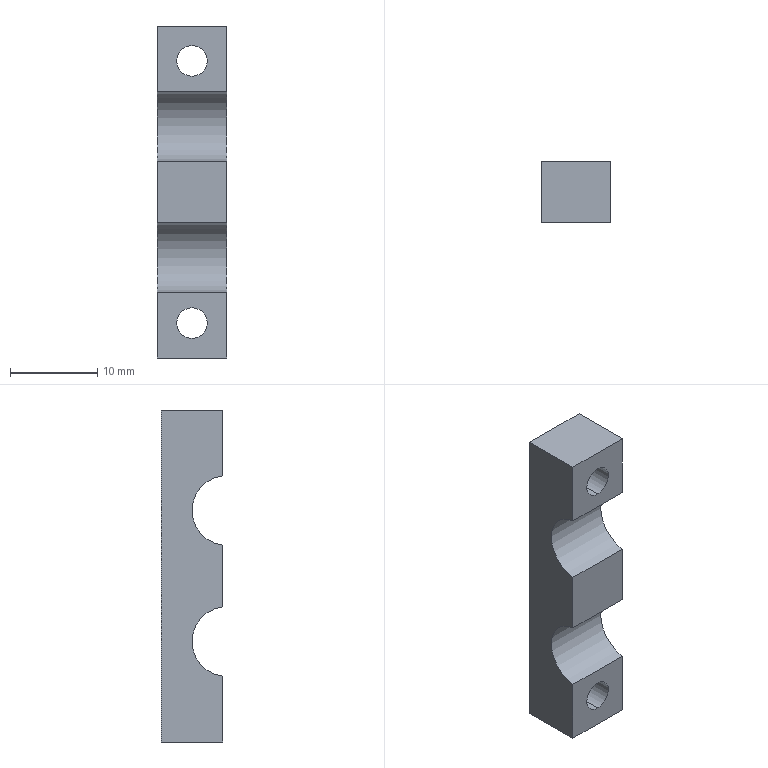Part | STEP file | 0246_216_Block | 1 solid | 20 faces | box 8 x 7 x 38 mm | volume 1490 mm3 | cylinder 10 | plane 10 | commonest cylinder face diameters 3.5 x4 6.5 x4 8 x2
STEP:
#1=CARTESIAN_POINT('',(0.,0.,0.));
#2=DIRECTION('',(0.,0.,1.));
#3=DIRECTION('',(1.,0.,0.));
#4=AXIS2_PLACEMENT_3D('',#1,#2,#3);
#5=CARTESIAN_POINT('',(0.,3.5,18.25));
#6=VERTEX_POINT('',#5);
#7=CARTESIAN_POINT('',(0.,7.,18.25));
#8=VERTEX_POINT('',#7);
#9=CARTESIAN_POINT('',(0.,7.,18.25));
#10=DIRECTION('',(0.,1.,0.));
#11=VECTOR('',#10,1.);
#12=LINE('',#9,#11);
#13=CARTESIAN_POINT('',(0.,7.,15.));
#14=DIRECTION('',(0.,1.,0.));
#15=DIRECTION('',(0.,0.,1.));
#16=AXIS2_PLACEMENT_3D('',#13,#14,#15);
#17=CYLINDRICAL_SURFACE('',#16,3.25);
#18=CARTESIAN_POINT('',(6.283,0.));
#19=DIRECTION('',(0.,1.));
#20=VECTOR('',#19,1.);
#21=LINE('',#18,#20);
#22=(GEOMETRIC_REPRESENTATION_CONTEXT(2)PARAMETRIC_REPRESENTATION_CONTEXT()REPRESENTATION_CONTEXT('',''));
#23=DEFINITIONAL_REPRESENTATION('',(#21),#22);
#24=PCURVE('',#17,#23);
#25=CARTESIAN_POINT('',(0.,7.,15.));
#26=DIRECTION('',(0.,1.,0.));
#27=DIRECTION('',(0.,0.,1.));
#28=AXIS2_PLACEMENT_3D('',#25,#26,#27);
#29=CYLINDRICAL_SURFACE('',#28,3.25);
#30=CARTESIAN_POINT('',(0.,0.));
#31=DIRECTION('',(0.,1.));
#32=VECTOR('',#31,1.);
#33=LINE('',#30,#32);
#34=(GEOMETRIC_REPRESENTATION_CONTEXT(2)PARAMETRIC_REPRESENTATION_CONTEXT()REPRESENTATION_CONTEXT('',''));
#35=DEFINITIONAL_REPRESENTATION('',(#33),#34);
#36=PCURVE('',#29,#35);
#37=SURFACE_CURVE('',#12,(#24,#36),.PCURVE_S1.);
#38=EDGE_CURVE('',#6,#8,#37,.T.);
#39=ORIENTED_EDGE('',*,*,#38,.T.);
#40=CARTESIAN_POINT('',(0.,7.,11.75));
#41=VERTEX_POINT('',#40);
#42=CARTESIAN_POINT('',(0.,7.,15.));
#43=DIRECTION('',(0.,1.,0.));
#44=DIRECTION('',(0.,0.,1.));
#45=AXIS2_PLACEMENT_3D('',#42,#43,#44);
#46=CIRCLE('',#45,3.25);
#47=CARTESIAN_POINT('',(0.,0.));
#48=DIRECTION('',(1.,0.));
#49=VECTOR('',#48,1.);
#50=LINE('',#47,#49);
#51=(GEOMETRIC_REPRESENTATION_CONTEXT(2)PARAMETRIC_REPRESENTATION_CONTEXT()REPRESENTATION_CONTEXT('',''));
#52=DEFINITIONAL_REPRESENTATION('',(#50),#51);
#53=PCURVE('',#17,#52);
#54=CARTESIAN_POINT('',(4.,7.,19.));
#55=DIRECTION('',(0.,-1.,0.));
#56=DIRECTION('',(0.,0.,-1.));
#57=AXIS2_PLACEMENT_3D('',#54,#55,#56);
#58=PLANE('',#57);
#59=CARTESIAN_POINT('',(0.75,-4.));
#60=CARTESIAN_POINT('',(0.75,1.629));
#61=CARTESIAN_POINT('',(5.625,-1.185));
#62=CARTESIAN_POINT('',(10.5,-4.));
#63=CARTESIAN_POINT('',(5.625,-6.815));
#64=CARTESIAN_POINT('',(0.75,-9.629));
#65=CARTESIAN_POINT('',(0.75,-4.));
#66=(BOUNDED_CURVE()B_SPLINE_CURVE(2,(#59,#60,#61,#62,#63,#64,#65),.UNSPECIFIED.,.T.,.F.)B_SPLINE_CURVE_WITH_KNOTS((1,2,2,2,2,1),(-2.094,0.,2.094,4.189,6.283,8.378),.UNSPECIFIED.)CURVE()GEOMETRIC_REPRESENTATION_ITEM()RATIONAL_B_SPLINE_CURVE((1.,0.5,1.,0.5,1.,0.5,1.))REPRESENTATION_ITEM(''));
#67=(GEOMETRIC_REPRESENTATION_CONTEXT(2)PARAMETRIC_REPRESENTATION_CONTEXT()REPRESENTATION_CONTEXT('',''));
#68=DEFINITIONAL_REPRESENTATION('',(#66),#67);
#69=PCURVE('',#58,#68);
#70=SURFACE_CURVE('',#46,(#53,#69),.PCURVE_S1.);
#71=EDGE_CURVE('',#41,#8,#70,.T.);
#72=ORIENTED_EDGE('',*,*,#71,.F.);
#73=CARTESIAN_POINT('',(0.,3.5,11.75));
#74=VERTEX_POINT('',#73);
#75=CARTESIAN_POINT('',(0.,7.,11.75));
#76=DIRECTION('',(0.,1.,0.));
#77=VECTOR('',#76,1.);
#78=LINE('',#75,#77);
#79=CARTESIAN_POINT('',(3.142,0.));
#80=DIRECTION('',(0.,1.));
#81=VECTOR('',#80,1.);
#82=LINE('',#79,#81);
#83=(GEOMETRIC_REPRESENTATION_CONTEXT(2)PARAMETRIC_REPRESENTATION_CONTEXT()REPRESENTATION_CONTEXT('',''));
#84=DEFINITIONAL_REPRESENTATION('',(#82),#83);
#85=PCURVE('',#17,#84);
#86=CARTESIAN_POINT('',(3.142,0.));
#87=DIRECTION('',(0.,1.));
#88=VECTOR('',#87,1.);
#89=LINE('',#86,#88);
#90=(GEOMETRIC_REPRESENTATION_CONTEXT(2)PARAMETRIC_REPRESENTATION_CONTEXT()REPRESENTATION_CONTEXT('',''));
#91=DEFINITIONAL_REPRESENTATION('',(#89),#90);
#92=PCURVE('',#29,#91);
#93=SURFACE_CURVE('',#78,(#85,#92),.PCURVE_S1.);
#94=EDGE_CURVE('',#74,#41,#93,.T.);
#95=ORIENTED_EDGE('',*,*,#94,.F.);
#96=CARTESIAN_POINT('',(0.,3.5,15.));
#97=DIRECTION('',(0.,1.,0.));
#98=DIRECTION('',(0.,0.,1.));
#99=AXIS2_PLACEMENT_3D('',#96,#97,#98);
#100=CIRCLE('',#99,3.25);
#101=CARTESIAN_POINT('',(0.,-3.5));
#102=DIRECTION('',(1.,0.));
#103=VECTOR('',#102,1.);
#104=LINE('',#101,#103);
#105=(GEOMETRIC_REPRESENTATION_CONTEXT(2)PARAMETRIC_REPRESENTATION_CONTEXT()REPRESENTATION_CONTEXT('',''));
#106=DEFINITIONAL_REPRESENTATION('',(#104),#105);
#107=PCURVE('',#17,#106);
#108=CARTESIAN_POINT('',(1.75,3.5,15.));
#109=DIRECTION('',(0.,-1.,0.));
#110=DIRECTION('',(0.,0.,-1.));
#111=AXIS2_PLACEMENT_3D('',#108,#109,#110);
#112=PLANE('',#111);
#113=CARTESIAN_POINT('',(-3.25,-1.75));
#114=CARTESIAN_POINT('',(-3.25,3.879));
#115=CARTESIAN_POINT('',(1.625,1.065));
#116=CARTESIAN_POINT('',(6.5,-1.75));
#117=CARTESIAN_POINT('',(1.625,-4.565));
#118=CARTESIAN_POINT('',(-3.25,-7.379));
#119=CARTESIAN_POINT('',(-3.25,-1.75));
#120=(BOUNDED_CURVE()B_SPLINE_CURVE(2,(#113,#114,#115,#116,#117,#118,#119),.UNSPECIFIED.,.T.,.F.)B_SPLINE_CURVE_WITH_KNOTS((1,2,2,2,2,1),(-2.094,0.,2.094,4.189,6.283,8.378),.UNSPECIFIED.)CURVE()GEOMETRIC_REPRESENTATION_ITEM()RATIONAL_B_SPLINE_CURVE((1.,0.5,1.,0.5,1.,0.5,1.))REPRESENTATION_ITEM(''));
#121=(GEOMETRIC_REPRESENTATION_CONTEXT(2)PARAMETRIC_REPRESENTATION_CONTEXT()REPRESENTATION_CONTEXT('',''));
#122=DEFINITIONAL_REPRESENTATION('',(#120),#121);
#123=PCURVE('',#112,#122);
#124=SURFACE_CURVE('',#100,(#107,#123),.PCURVE_S1.);
#125=EDGE_CURVE('',#74,#6,#124,.T.);
#126=ORIENTED_EDGE('',*,*,#125,.T.);
#127=EDGE_LOOP('',(#39,#72,#95,#126));
#128=FACE_BOUND('',#127,.F.);
#129=ADVANCED_FACE('',(#128),#17,.F.);
#130=CARTESIAN_POINT('',(0.,0.,16.75));
#131=VERTEX_POINT('',#130);
#132=CARTESIAN_POINT('',(0.,3.5,16.75));
#133=VERTEX_POINT('',#132);
#134=CARTESIAN_POINT('',(0.,7.,16.75));
#135=DIRECTION('',(0.,1.,0.));
#136=VECTOR('',#135,1.);
#137=LINE('',#134,#136);
#138=CARTESIAN_POINT('',(0.,7.,15.));
#139=DIRECTION('',(0.,1.,0.));
#140=DIRECTION('',(0.,0.,1.));
#141=AXIS2_PLACEMENT_3D('',#138,#139,#140);
#142=CYLINDRICAL_SURFACE('',#141,1.75);
#143=CARTESIAN_POINT('',(6.283,0.));
#144=DIRECTION('',(0.,1.));
#145=VECTOR('',#144,1.);
#146=LINE('',#143,#145);
#147=(GEOMETRIC_REPRESENTATION_CONTEXT(2)PARAMETRIC_REPRESENTATION_CONTEXT()REPRESENTATION_CONTEXT('',''));
#148=DEFINITIONAL_REPRESENTATION('',(#146),#147);
#149=PCURVE('',#142,#148);
#150=CARTESIAN_POINT('',(0.,7.,15.));
#151=DIRECTION('',(0.,1.,0.));
#152=DIRECTION('',(0.,0.,1.));
#153=AXIS2_PLACEMENT_3D('',#150,#151,#152);
#154=CYLINDRICAL_SURFACE('',#153,1.75);
#155=CARTESIAN_POINT('',(0.,0.));
#156=DIRECTION('',(0.,1.));
#157=VECTOR('',#156,1.);
#158=LINE('',#155,#157);
#159=(GEOMETRIC_REPRESENTATION_CONTEXT(2)PARAMETRIC_REPRESENTATION_CONTEXT()REPRESENTATION_CONTEXT('',''));
#160=DEFINITIONAL_REPRESENTATION('',(#158),#159);
#161=PCURVE('',#154,#160);
#162=SURFACE_CURVE('',#137,(#149,#161),.PCURVE_S1.);
#163=EDGE_CURVE('',#131,#133,#162,.T.);
#164=ORIENTED_EDGE('',*,*,#163,.T.);
#165=CARTESIAN_POINT('',(0.,3.5,13.25));
#166=VERTEX_POINT('',#165);
#167=CARTESIAN_POINT('',(0.,3.5,15.));
#168=DIRECTION('',(0.,1.,0.));
#169=DIRECTION('',(0.,0.,1.));
#170=AXIS2_PLACEMENT_3D('',#167,#168,#169);
#171=CIRCLE('',#170,1.75);
#172=CARTESIAN_POINT('',(0.,-3.5));
#173=DIRECTION('',(1.,0.));
#174=VECTOR('',#173,1.);
#175=LINE('',#172,#174);
#176=(GEOMETRIC_REPRESENTATION_CONTEXT(2)PARAMETRIC_REPRESENTATION_CONTEXT()REPRESENTATION_CONTEXT('',''));
#177=DEFINITIONAL_REPRESENTATION('',(#175),#176);
#178=PCURVE('',#142,#177);
#179=CARTESIAN_POINT('',(-1.75,-1.75));
#180=CARTESIAN_POINT('',(-1.75,1.281));
#181=CARTESIAN_POINT('',(0.875,-0.2345));
#182=CARTESIAN_POINT('',(3.5,-1.75));
#183=CARTESIAN_POINT('',(0.875,-3.266));
#184=CARTESIAN_POINT('',(-1.75,-4.781));
#185=CARTESIAN_POINT('',(-1.75,-1.75));
#186=(BOUNDED_CURVE()B_SPLINE_CURVE(2,(#179,#180,#181,#182,#183,#184,#185),.UNSPECIFIED.,.T.,.F.)B_SPLINE_CURVE_WITH_KNOTS((1,2,2,2,2,1),(-2.094,0.,2.094,4.189,6.283,8.378),.UNSPECIFIED.)CURVE()GEOMETRIC_REPRESENTATION_ITEM()RATIONAL_B_SPLINE_CURVE((1.,0.5,1.,0.5,1.,0.5,1.))REPRESENTATION_ITEM(''));
#187=(GEOMETRIC_REPRESENTATION_CONTEXT(2)PARAMETRIC_REPRESENTATION_CONTEXT()REPRESENTATION_CONTEXT('',''));
#188=DEFINITIONAL_REPRESENTATION('',(#186),#187);
#189=PCURVE('',#112,#188);
#190=SURFACE_CURVE('',#171,(#178,#189),.PCURVE_S1.);
#191=EDGE_CURVE('',#166,#133,#190,.T.);
#192=ORIENTED_EDGE('',*,*,#191,.F.);
#193=CARTESIAN_POINT('',(0.,0.,13.25));
#194=VERTEX_POINT('',#193);
#195=CARTESIAN_POINT('',(0.,7.,13.25));
#196=DIRECTION('',(0.,1.,0.));
#197=VECTOR('',#196,1.);
#198=LINE('',#195,#197);
#199=CARTESIAN_POINT('',(3.142,0.));
#200=DIRECTION('',(0.,1.));
#201=VECTOR('',#200,1.);
#202=LINE('',#199,#201);
#203=(GEOMETRIC_REPRESENTATION_CONTEXT(2)PARAMETRIC_REPRESENTATION_CONTEXT()REPRESENTATION_CONTEXT('',''));
#204=DEFINITIONAL_REPRESENTATION('',(#202),#203);
#205=PCURVE('',#142,#204);
#206=CARTESIAN_POINT('',(3.142,0.));
#207=DIRECTION('',(0.,1.));
#208=VECTOR('',#207,1.);
#209=LINE('',#206,#208);
#210=(GEOMETRIC_REPRESENTATION_CONTEXT(2)PARAMETRIC_REPRESENTATION_CONTEXT()REPRESENTATION_CONTEXT('',''));
#211=DEFINITIONAL_REPRESENTATION('',(#209),#210);
#212=PCURVE('',#154,#211);
#213=SURFACE_CURVE('',#198,(#205,#212),.PCURVE_S1.);
#214=EDGE_CURVE('',#194,#166,#213,.T.);
#215=ORIENTED_EDGE('',*,*,#214,.F.);
#216=CARTESIAN_POINT('',(0.,0.,15.));
#217=DIRECTION('',(0.,1.,0.));
#218=DIRECTION('',(0.,0.,1.));
#219=AXIS2_PLACEMENT_3D('',#216,#217,#218);
#220=CIRCLE('',#219,1.75);
#221=CARTESIAN_POINT('',(0.,-7.));
#222=DIRECTION('',(1.,0.));
#223=VECTOR('',#222,1.);
#224=LINE('',#221,#223);
#225=(GEOMETRIC_REPRESENTATION_CONTEXT(2)PARAMETRIC_REPRESENTATION_CONTEXT()REPRESENTATION_CONTEXT('',''));
#226=DEFINITIONAL_REPRESENTATION('',(#224),#225);
#227=PCURVE('',#142,#226);
#228=CARTESIAN_POINT('',(4.,0.,19.));
#229=DIRECTION('',(0.,1.,0.));
#230=DIRECTION('',(0.,0.,1.));
#231=AXIS2_PLACEMENT_3D('',#228,#229,#230);
#232=PLANE('',#231);
#233=CARTESIAN_POINT('',(-4.,-4.));
#234=DIRECTION('',(1.,0.));
#235=AXIS2_PLACEMENT_2D('',#233,#234);
#236=CIRCLE('',#235,1.75);
#237=(GEOMETRIC_REPRESENTATION_CONTEXT(2)PARAMETRIC_REPRESENTATION_CONTEXT()REPRESENTATION_CONTEXT('',''));
#238=DEFINITIONAL_REPRESENTATION('',(#236),#237);
#239=PCURVE('',#232,#238);
#240=SURFACE_CURVE('',#220,(#227,#239),.PCURVE_S1.);
#241=EDGE_CURVE('',#194,#131,#240,.T.);
#242=ORIENTED_EDGE('',*,*,#241,.T.);
#243=EDGE_LOOP('',(#164,#192,#215,#242));
#244=FACE_BOUND('',#243,.F.);
#245=ADVANCED_FACE('',(#244),#142,.F.);
#246=CARTESIAN_POINT('',(0.,3.5,-11.75));
#247=VERTEX_POINT('',#246);
#248=CARTESIAN_POINT('',(0.,7.,-11.75));
#249=VERTEX_POINT('',#248);
#250=CARTESIAN_POINT('',(0.,7.,-11.75));
#251=DIRECTION('',(0.,1.,0.));
#252=VECTOR('',#251,1.);
#253=LINE('',#250,#252);
#254=CARTESIAN_POINT('',(0.,7.,-15.));
#255=DIRECTION('',(0.,1.,0.));
#256=DIRECTION('',(0.,0.,1.));
#257=AXIS2_PLACEMENT_3D('',#254,#255,#256);
#258=CYLINDRICAL_SURFACE('',#257,3.25);
#259=CARTESIAN_POINT('',(6.283,0.));
#260=DIRECTION('',(0.,1.));
#261=VECTOR('',#260,1.);
#262=LINE('',#259,#261);
#263=(GEOMETRIC_REPRESENTATION_CONTEXT(2)PARAMETRIC_REPRESENTATION_CONTEXT()REPRESENTATION_CONTEXT('',''));
#264=DEFINITIONAL_REPRESENTATION('',(#262),#263);
#265=PCURVE('',#258,#264);
#266=CARTESIAN_POINT('',(0.,7.,-15.));
#267=DIRECTION('',(0.,1.,0.));
#268=DIRECTION('',(0.,0.,1.));
#269=AXIS2_PLACEMENT_3D('',#266,#267,#268);
#270=CYLINDRICAL_SURFACE('',#269,3.25);
#271=CARTESIAN_POINT('',(0.,0.));
#272=DIRECTION('',(0.,1.));
#273=VECTOR('',#272,1.);
#274=LINE('',#271,#273);
#275=(GEOMETRIC_REPRESENTATION_CONTEXT(2)PARAMETRIC_REPRESENTATION_CONTEXT()REPRESENTATION_CONTEXT('',''));
#276=DEFINITIONAL_REPRESENTATION('',(#274),#275);
#277=PCURVE('',#270,#276);
#278=SURFACE_CURVE('',#253,(#265,#277),.PCURVE_S1.);
#279=EDGE_CURVE('',#247,#249,#278,.T.);
#280=ORIENTED_EDGE('',*,*,#279,.T.);
#281=CARTESIAN_POINT('',(0.,7.,-18.25));
#282=VERTEX_POINT('',#281);
#283=CARTESIAN_POINT('',(0.,7.,-15.));
#284=DIRECTION('',(0.,1.,0.));
#285=DIRECTION('',(0.,0.,1.));
#286=AXIS2_PLACEMENT_3D('',#283,#284,#285);
#287=CIRCLE('',#286,3.25);
#288=CARTESIAN_POINT('',(0.,0.));
#289=DIRECTION('',(1.,0.));
#290=VECTOR('',#289,1.);
#291=LINE('',#288,#290);
#292=(GEOMETRIC_REPRESENTATION_CONTEXT(2)PARAMETRIC_REPRESENTATION_CONTEXT()REPRESENTATION_CONTEXT('',''));
#293=DEFINITIONAL_REPRESENTATION('',(#291),#292);
#294=PCURVE('',#258,#293);
#295=CARTESIAN_POINT('',(30.75,-4.));
#296=CARTESIAN_POINT('',(30.75,1.629));
#297=CARTESIAN_POINT('',(35.625,-1.185));
#298=CARTESIAN_POINT('',(40.5,-4.));
#299=CARTESIAN_POINT('',(35.625,-6.815));
#300=CARTESIAN_POINT('',(30.75,-9.629));
#301=CARTESIAN_POINT('',(30.75,-4.));
#302=(BOUNDED_CURVE()B_SPLINE_CURVE(2,(#295,#296,#297,#298,#299,#300,#301),.UNSPECIFIED.,.T.,.F.)B_SPLINE_CURVE_WITH_KNOTS((1,2,2,2,2,1),(-2.094,0.,2.094,4.189,6.283,8.378),.UNSPECIFIED.)CURVE()GEOMETRIC_REPRESENTATION_ITEM()RATIONAL_B_SPLINE_CURVE((1.,0.5,1.,0.5,1.,0.5,1.))REPRESENTATION_ITEM(''));
#303=(GEOMETRIC_REPRESENTATION_CONTEXT(2)PARAMETRIC_REPRESENTATION_CONTEXT()REPRESENTATION_CONTEXT('',''));
#304=DEFINITIONAL_REPRESENTATION('',(#302),#303);
#305=PCURVE('',#58,#304);
#306=SURFACE_CURVE('',#287,(#294,#305),.PCURVE_S1.);
#307=EDGE_CURVE('',#282,#249,#306,.T.);
#308=ORIENTED_EDGE('',*,*,#307,.F.);
#309=CARTESIAN_POINT('',(0.,3.5,-18.25));
#310=VERTEX_POINT('',#309);
#311=CARTESIAN_POINT('',(0.,7.,-18.25));
#312=DIRECTION('',(0.,1.,0.));
#313=VECTOR('',#312,1.);
#314=LINE('',#311,#313);
#315=CARTESIAN_POINT('',(3.142,0.));
#316=DIRECTION('',(0.,1.));
#317=VECTOR('',#316,1.);
#318=LINE('',#315,#317);
#319=(GEOMETRIC_REPRESENTATION_CONTEXT(2)PARAMETRIC_REPRESENTATION_CONTEXT()REPRESENTATION_CONTEXT('',''));
#320=DEFINITIONAL_REPRESENTATION('',(#318),#319);
#321=PCURVE('',#258,#320);
#322=CARTESIAN_POINT('',(3.142,0.));
#323=DIRECTION('',(0.,1.));
#324=VECTOR('',#323,1.);
#325=LINE('',#322,#324);
#326=(GEOMETRIC_REPRESENTATION_CONTEXT(2)PARAMETRIC_REPRESENTATION_CONTEXT()REPRESENTATION_CONTEXT('',''));
#327=DEFINITIONAL_REPRESENTATION('',(#325),#326);
#328=PCURVE('',#270,#327);
#329=SURFACE_CURVE('',#314,(#321,#328),.PCURVE_S1.);
#330=EDGE_CURVE('',#310,#282,#329,.T.);
#331=ORIENTED_EDGE('',*,*,#330,.F.);
#332=CARTESIAN_POINT('',(0.,3.5,-15.));
#333=DIRECTION('',(0.,1.,0.));
#334=DIRECTION('',(0.,0.,1.));
#335=AXIS2_PLACEMENT_3D('',#332,#333,#334);
#336=CIRCLE('',#335,3.25);
#337=CARTESIAN_POINT('',(0.,-3.5));
#338=DIRECTION('',(1.,0.));
#339=VECTOR('',#338,1.);
#340=LINE('',#337,#339);
#341=(GEOMETRIC_REPRESENTATION_CONTEXT(2)PARAMETRIC_REPRESENTATION_CONTEXT()REPRESENTATION_CONTEXT('',''));
#342=DEFINITIONAL_REPRESENTATION('',(#340),#341);
#343=PCURVE('',#258,#342);
#344=CARTESIAN_POINT('',(1.75,3.5,-15.));
#345=DIRECTION('',(0.,-1.,0.));
#346=DIRECTION('',(0.,0.,-1.));
#347=AXIS2_PLACEMENT_3D('',#344,#345,#346);
#348=PLANE('',#347);
#349=CARTESIAN_POINT('',(-3.25,-1.75));
#350=CARTESIAN_POINT('',(-3.25,3.879));
#351=CARTESIAN_POINT('',(1.625,1.065));
#352=CARTESIAN_POINT('',(6.5,-1.75));
#353=CARTESIAN_POINT('',(1.625,-4.565));
#354=CARTESIAN_POINT('',(-3.25,-7.379));
#355=CARTESIAN_POINT('',(-3.25,-1.75));
#356=(BOUNDED_CURVE()B_SPLINE_CURVE(2,(#349,#350,#351,#352,#353,#354,#355),.UNSPECIFIED.,.T.,.F.)B_SPLINE_CURVE_WITH_KNOTS((1,2,2,2,2,1),(-2.094,0.,2.094,4.189,6.283,8.378),.UNSPECIFIED.)CURVE()GEOMETRIC_REPRESENTATION_ITEM()RATIONAL_B_SPLINE_CURVE((1.,0.5,1.,0.5,1.,0.5,1.))REPRESENTATION_ITEM(''));
#357=(GEOMETRIC_REPRESENTATION_CONTEXT(2)PARAMETRIC_REPRESENTATION_CONTEXT()REPRESENTATION_CONTEXT('',''));
#358=DEFINITIONAL_REPRESENTATION('',(#356),#357);
#359=PCURVE('',#348,#358);
#360=SURFACE_CURVE('',#336,(#343,#359),.PCURVE_S1.);
#361=EDGE_CURVE('',#310,#247,#360,.T.);
#362=ORIENTED_EDGE('',*,*,#361,.T.);
#363=EDGE_LOOP('',(#280,#308,#331,#362));
#364=FACE_BOUND('',#363,.F.);
#365=ADVANCED_FACE('',(#364),#258,.F.);
#366=CARTESIAN_POINT('',(0.,0.,-13.25));
#367=VERTEX_POINT('',#366);
#368=CARTESIAN_POINT('',(0.,3.5,-13.25));
#369=VERTEX_POINT('',#368);
#370=CARTESIAN_POINT('',(0.,7.,-13.25));
#371=DIRECTION('',(0.,1.,0.));
#372=VECTOR('',#371,1.);
#373=LINE('',#370,#372);
#374=CARTESIAN_POINT('',(0.,7.,-15.));
#375=DIRECTION('',(0.,1.,0.));
#376=DIRECTION('',(0.,0.,1.));
#377=AXIS2_PLACEMENT_3D('',#374,#375,#376);
#378=CYLINDRICAL_SURFACE('',#377,1.75);
#379=CARTESIAN_POINT('',(6.283,0.));
#380=DIRECTION('',(0.,1.));
#381=VECTOR('',#380,1.);
#382=LINE('',#379,#381);
#383=(GEOMETRIC_REPRESENTATION_CONTEXT(2)PARAMETRIC_REPRESENTATION_CONTEXT()REPRESENTATION_CONTEXT('',''));
#384=DEFINITIONAL_REPRESENTATION('',(#382),#383);
#385=PCURVE('',#378,#384);
#386=CARTESIAN_POINT('',(0.,7.,-15.));
#387=DIRECTION('',(0.,1.,0.));
#388=DIRECTION('',(0.,0.,1.));
#389=AXIS2_PLACEMENT_3D('',#386,#387,#388);
#390=CYLINDRICAL_SURFACE('',#389,1.75);
#391=CARTESIAN_POINT('',(0.,0.));
#392=DIRECTION('',(0.,1.));
#393=VECTOR('',#392,1.);
#394=LINE('',#391,#393);
#395=(GEOMETRIC_REPRESENTATION_CONTEXT(2)PARAMETRIC_REPRESENTATION_CONTEXT()REPRESENTATION_CONTEXT('',''));
#396=DEFINITIONAL_REPRESENTATION('',(#394),#395);
#397=PCURVE('',#390,#396);
#398=SURFACE_CURVE('',#373,(#385,#397),.PCURVE_S1.);
#399=EDGE_CURVE('',#367,#369,#398,.T.);
#400=ORIENTED_EDGE('',*,*,#399,.T.);
#401=CARTESIAN_POINT('',(0.,3.5,-16.75));
#402=VERTEX_POINT('',#401);
#403=CARTESIAN_POINT('',(0.,3.5,-15.));
#404=DIRECTION('',(0.,1.,0.));
#405=DIRECTION('',(0.,0.,1.));
#406=AXIS2_PLACEMENT_3D('',#403,#404,#405);
#407=CIRCLE('',#406,1.75);
#408=CARTESIAN_POINT('',(0.,-3.5));
#409=DIRECTION('',(1.,0.));
#410=VECTOR('',#409,1.);
#411=LINE('',#408,#410);
#412=(GEOMETRIC_REPRESENTATION_CONTEXT(2)PARAMETRIC_REPRESENTATION_CONTEXT()REPRESENTATION_CONTEXT('',''));
#413=DEFINITIONAL_REPRESENTATION('',(#411),#412);
#414=PCURVE('',#378,#413);
#415=CARTESIAN_POINT('',(-1.75,-1.75));
#416=CARTESIAN_POINT('',(-1.75,1.281));
#417=CARTESIAN_POINT('',(0.875,-0.2345));
#418=CARTESIAN_POINT('',(3.5,-1.75));
#419=CARTESIAN_POINT('',(0.875,-3.266));
#420=CARTESIAN_POINT('',(-1.75,-4.781));
#421=CARTESIAN_POINT('',(-1.75,-1.75));
#422=(BOUNDED_CURVE()B_SPLINE_CURVE(2,(#415,#416,#417,#418,#419,#420,#421),.UNSPECIFIED.,.T.,.F.)B_SPLINE_CURVE_WITH_KNOTS((1,2,2,2,2,1),(-2.094,0.,2.094,4.189,6.283,8.378),.UNSPECIFIED.)CURVE()GEOMETRIC_REPRESENTATION_ITEM()RATIONAL_B_SPLINE_CURVE((1.,0.5,1.,0.5,1.,0.5,1.))REPRESENTATION_ITEM(''));
#423=(GEOMETRIC_REPRESENTATION_CONTEXT(2)PARAMETRIC_REPRESENTATION_CONTEXT()REPRESENTATION_CONTEXT('',''));
#424=DEFINITIONAL_REPRESENTATION('',(#422),#423);
#425=PCURVE('',#348,#424);
#426=SURFACE_CURVE('',#407,(#414,#425),.PCURVE_S1.);
#427=EDGE_CURVE('',#402,#369,#426,.T.);
#428=ORIENTED_EDGE('',*,*,#427,.F.);
#429=CARTESIAN_POINT('',(0.,0.,-16.75));
#430=VERTEX_POINT('',#429);
#431=CARTESIAN_POINT('',(0.,7.,-16.75));
#432=DIRECTION('',(0.,1.,0.));
#433=VECTOR('',#432,1.);
#434=LINE('',#431,#433);
#435=CARTESIAN_POINT('',(3.142,0.));
#436=DIRECTION('',(0.,1.));
#437=VECTOR('',#436,1.);
#438=LINE('',#435,#437);
#439=(GEOMETRIC_REPRESENTATION_CONTEXT(2)PARAMETRIC_REPRESENTATION_CONTEXT()REPRESENTATION_CONTEXT('',''));
#440=DEFINITIONAL_REPRESENTATION('',(#438),#439);
#441=PCURVE('',#378,#440);
#442=CARTESIAN_POINT('',(3.142,0.));
#443=DIRECTION('',(0.,1.));
#444=VECTOR('',#443,1.);
#445=LINE('',#442,#444);
#446=(GEOMETRIC_REPRESENTATION_CONTEXT(2)PARAMETRIC_REPRESENTATION_CONTEXT()REPRESENTATION_CONTEXT('',''));
#447=DEFINITIONAL_REPRESENTATION('',(#445),#446);
#448=PCURVE('',#390,#447);
#449=SURFACE_CURVE('',#434,(#441,#448),.PCURVE_S1.);
#450=EDGE_CURVE('',#430,#402,#449,.T.);
#451=ORIENTED_EDGE('',*,*,#450,.F.);
#452=CARTESIAN_POINT('',(0.,0.,-15.));
#453=DIRECTION('',(0.,1.,0.));
#454=DIRECTION('',(0.,0.,1.));
#455=AXIS2_PLACEMENT_3D('',#452,#453,#454);
#456=CIRCLE('',#455,1.75);
#457=CARTESIAN_POINT('',(0.,-7.));
#458=DIRECTION('',(1.,0.));
#459=VECTOR('',#458,1.);
#460=LINE('',#457,#459);
#461=(GEOMETRIC_REPRESENTATION_CONTEXT(2)PARAMETRIC_REPRESENTATION_CONTEXT()REPRESENTATION_CONTEXT('',''));
#462=DEFINITIONAL_REPRESENTATION('',(#460),#461);
#463=PCURVE('',#378,#462);
#464=CARTESIAN_POINT('',(4.,0.,-11.469));
#465=DIRECTION('',(0.,1.,0.));
#466=DIRECTION('',(0.,0.,1.));
#467=AXIS2_PLACEMENT_3D('',#464,#465,#466);
#468=PLANE('',#467);
#469=CARTESIAN_POINT('',(-3.531,-4.));
#470=DIRECTION('',(1.,0.));
#471=AXIS2_PLACEMENT_2D('',#469,#470);
#472=CIRCLE('',#471,1.75);
#473=(GEOMETRIC_REPRESENTATION_CONTEXT(2)PARAMETRIC_REPRESENTATION_CONTEXT()REPRESENTATION_CONTEXT('',''));
#474=DEFINITIONAL_REPRESENTATION('',(#472),#473);
#475=PCURVE('',#468,#474);
#476=SURFACE_CURVE('',#456,(#463,#475),.PCURVE_S1.);
#477=EDGE_CURVE('',#430,#367,#476,.T.);
#478=ORIENTED_EDGE('',*,*,#477,.T.);
#479=EDGE_LOOP('',(#400,#428,#451,#478));
#480=FACE_BOUND('',#479,.F.);
#481=ADVANCED_FACE('',(#480),#378,.F.);
#482=CARTESIAN_POINT('',(0.,0.,15.));
#483=DIRECTION('',(0.,1.,0.));
#484=DIRECTION('',(0.,0.,1.));
#485=AXIS2_PLACEMENT_3D('',#482,#483,#484);
#486=CIRCLE('',#485,1.75);
#487=CARTESIAN_POINT('',(-4.,-4.));
#488=DIRECTION('',(1.,0.));
#489=AXIS2_PLACEMENT_2D('',#487,#488);
#490=CIRCLE('',#489,1.75);
#491=(GEOMETRIC_REPRESENTATION_CONTEXT(2)PARAMETRIC_REPRESENTATION_CONTEXT()REPRESENTATION_CONTEXT('',''));
#492=DEFINITIONAL_REPRESENTATION('',(#490),#491);
#493=PCURVE('',#232,#492);
#494=CARTESIAN_POINT('',(0.,-7.));
#495=DIRECTION('',(1.,0.));
#496=VECTOR('',#495,1.);
#497=LINE('',#494,#496);
#498=(GEOMETRIC_REPRESENTATION_CONTEXT(2)PARAMETRIC_REPRESENTATION_CONTEXT()REPRESENTATION_CONTEXT('',''));
#499=DEFINITIONAL_REPRESENTATION('',(#497),#498);
#500=PCURVE('',#154,#499);
#501=SURFACE_CURVE('',#486,(#493,#500),.PCURVE_S1.);
#502=EDGE_CURVE('',#131,#194,#501,.T.);
#503=ORIENTED_EDGE('',*,*,#502,.T.);
#504=ORIENTED_EDGE('',*,*,#241,.T.);
#505=EDGE_LOOP('',(#503,#504));
#506=FACE_BOUND('',#505,.T.);
#507=CARTESIAN_POINT('',(-4.,0.,19.));
#508=VERTEX_POINT('',#507);
#509=CARTESIAN_POINT('',(-4.,0.,11.469));
#510=VERTEX_POINT('',#509);
#511=CARTESIAN_POINT('',(-4.,0.,19.));
#512=DIRECTION('',(0.,0.,-1.));
#513=VECTOR('',#512,1.);
#514=LINE('',#511,#513);
#515=CARTESIAN_POINT('',(0.,-8.));
#516=DIRECTION('',(-1.,0.));
#517=VECTOR('',#516,1.);
#518=LINE('',#515,#517);
#519=(GEOMETRIC_REPRESENTATION_CONTEXT(2)PARAMETRIC_REPRESENTATION_CONTEXT()REPRESENTATION_CONTEXT('',''));
#520=DEFINITIONAL_REPRESENTATION('',(#518),#519);
#521=PCURVE('',#232,#520);
#522=CARTESIAN_POINT('',(-4.,-0.5,7.5));
#523=DIRECTION('',(-1.,0.,0.));
#524=DIRECTION('',(0.,0.,1.));
#525=AXIS2_PLACEMENT_3D('',#522,#523,#524);
#526=PLANE('',#525);
#527=CARTESIAN_POINT('',(11.5,0.5));
#528=DIRECTION('',(-1.,0.));
#529=VECTOR('',#528,1.);
#530=LINE('',#527,#529);
#531=(GEOMETRIC_REPRESENTATION_CONTEXT(2)PARAMETRIC_REPRESENTATION_CONTEXT()REPRESENTATION_CONTEXT('',''));
#532=DEFINITIONAL_REPRESENTATION('',(#530),#531);
#533=PCURVE('',#526,#532);
#534=SURFACE_CURVE('',#514,(#521,#533),.PCURVE_S1.);
#535=EDGE_CURVE('',#508,#510,#534,.T.);
#536=ORIENTED_EDGE('',*,*,#535,.T.);
#537=CARTESIAN_POINT('',(4.,0.,11.469));
#538=VERTEX_POINT('',#537);
#539=CARTESIAN_POINT('',(4.,0.,11.469));
#540=DIRECTION('',(-1.,0.,0.));
#541=VECTOR('',#540,1.);
#542=LINE('',#539,#541);
#543=CARTESIAN_POINT('',(-7.531,0.));
#544=DIRECTION('',(0.,-1.));
#545=VECTOR('',#544,1.);
#546=LINE('',#543,#545);
#547=(GEOMETRIC_REPRESENTATION_CONTEXT(2)PARAMETRIC_REPRESENTATION_CONTEXT()REPRESENTATION_CONTEXT('',''));
#548=DEFINITIONAL_REPRESENTATION('',(#546),#547);
#549=PCURVE('',#232,#548);
#550=CARTESIAN_POINT('',(4.,-0.5,7.5));
#551=DIRECTION('',(-1.,0.,0.));
#552=DIRECTION('',(0.,0.,1.));
#553=AXIS2_PLACEMENT_3D('',#550,#551,#552);
#554=CYLINDRICAL_SURFACE('',#553,4.);
#555=CARTESIAN_POINT('',(0.1253,0.));
#556=DIRECTION('',(0.,1.));
#557=VECTOR('',#556,1.);
#558=LINE('',#555,#557);
#559=(GEOMETRIC_REPRESENTATION_CONTEXT(2)PARAMETRIC_REPRESENTATION_CONTEXT()REPRESENTATION_CONTEXT('',''));
#560=DEFINITIONAL_REPRESENTATION('',(#558),#559);
#561=PCURVE('',#554,#560);
#562=SURFACE_CURVE('',#542,(#549,#561),.PCURVE_S1.);
#563=EDGE_CURVE('',#538,#510,#562,.T.);
#564=ORIENTED_EDGE('',*,*,#563,.F.);
#565=CARTESIAN_POINT('',(4.,0.,19.));
#566=VERTEX_POINT('',#565);
#567=CARTESIAN_POINT('',(4.,0.,19.));
#568=DIRECTION('',(0.,0.,-1.));
#569=VECTOR('',#568,1.);
#570=LINE('',#567,#569);
#571=CARTESIAN_POINT('',(0.,0.));
#572=DIRECTION('',(-1.,0.));
#573=VECTOR('',#572,1.);
#574=LINE('',#571,#573);
#575=(GEOMETRIC_REPRESENTATION_CONTEXT(2)PARAMETRIC_REPRESENTATION_CONTEXT()REPRESENTATION_CONTEXT('',''));
#576=DEFINITIONAL_REPRESENTATION('',(#574),#575);
#577=PCURVE('',#232,#576);
#578=CARTESIAN_POINT('',(4.,-0.5,7.5));
#579=DIRECTION('',(-1.,0.,0.));
#580=DIRECTION('',(0.,0.,1.));
#581=AXIS2_PLACEMENT_3D('',#578,#579,#580);
#582=PLANE('',#581);
#583=CARTESIAN_POINT('',(11.5,0.5));
#584=DIRECTION('',(-1.,0.));
#585=VECTOR('',#584,1.);
#586=LINE('',#583,#585);
#587=(GEOMETRIC_REPRESENTATION_CONTEXT(2)PARAMETRIC_REPRESENTATION_CONTEXT()REPRESENTATION_CONTEXT('',''));
#588=DEFINITIONAL_REPRESENTATION('',(#586),#587);
#589=PCURVE('',#582,#588);
#590=SURFACE_CURVE('',#570,(#577,#589),.PCURVE_S1.);
#591=EDGE_CURVE('',#566,#538,#590,.T.);
#592=ORIENTED_EDGE('',*,*,#591,.F.);
#593=CARTESIAN_POINT('',(4.,0.,19.));
#594=DIRECTION('',(-1.,0.,0.));
#595=VECTOR('',#594,1.);
#596=LINE('',#593,#595);
#597=CARTESIAN_POINT('',(0.,0.));
#598=DIRECTION('',(0.,-1.));
#599=VECTOR('',#598,1.);
#600=LINE('',#597,#599);
#601=(GEOMETRIC_REPRESENTATION_CONTEXT(2)PARAMETRIC_REPRESENTATION_CONTEXT()REPRESENTATION_CONTEXT('',''));
#602=DEFINITIONAL_REPRESENTATION('',(#600),#601);
#603=PCURVE('',#232,#602);
#604=CARTESIAN_POINT('',(4.,0.,19.));
#605=DIRECTION('',(0.,0.,-1.));
#606=DIRECTION('',(-1.,0.,0.));
#607=AXIS2_PLACEMENT_3D('',#604,#605,#606);
#608=PLANE('',#607);
#609=CARTESIAN_POINT('',(0.,0.));
#610=DIRECTION('',(1.,0.));
#611=VECTOR('',#610,1.);
#612=LINE('',#609,#611);
#613=(GEOMETRIC_REPRESENTATION_CONTEXT(2)PARAMETRIC_REPRESENTATION_CONTEXT()REPRESENTATION_CONTEXT('',''));
#614=DEFINITIONAL_REPRESENTATION('',(#612),#613);
#615=PCURVE('',#608,#614);
#616=SURFACE_CURVE('',#596,(#603,#615),.PCURVE_S1.);
#617=EDGE_CURVE('',#566,#508,#616,.T.);
#618=ORIENTED_EDGE('',*,*,#617,.T.);
#619=EDGE_LOOP('',(#536,#564,#592,#618));
#620=FACE_BOUND('',#619,.T.);
#621=ADVANCED_FACE('',(#506,#620),#232,.F.);
#622=ORIENTED_EDGE('',*,*,#563,.F.);
#623=CARTESIAN_POINT('',(4.,0.,3.531));
#624=VERTEX_POINT('',#623);
#625=CARTESIAN_POINT('',(4.,-0.5,7.5));
#626=DIRECTION('',(-1.,0.,0.));
#627=DIRECTION('',(0.,0.,1.));
#628=AXIS2_PLACEMENT_3D('',#625,#626,#627);
#629=CIRCLE('',#628,4.);
#630=CARTESIAN_POINT('',(0.,0.));
#631=DIRECTION('',(1.,0.));
#632=VECTOR('',#631,1.);
#633=LINE('',#630,#632);
#634=(GEOMETRIC_REPRESENTATION_CONTEXT(2)PARAMETRIC_REPRESENTATION_CONTEXT()REPRESENTATION_CONTEXT('',''));
#635=DEFINITIONAL_REPRESENTATION('',(#633),#634);
#636=PCURVE('',#554,#635);
#637=CARTESIAN_POINT('',(0.,0.));
#638=DIRECTION('',(1.,0.));
#639=AXIS2_PLACEMENT_2D('',#637,#638);
#640=CIRCLE('',#639,4.);
#641=(GEOMETRIC_REPRESENTATION_CONTEXT(2)PARAMETRIC_REPRESENTATION_CONTEXT()REPRESENTATION_CONTEXT('',''));
#642=DEFINITIONAL_REPRESENTATION('',(#640),#641);
#643=PCURVE('',#582,#642);
#644=SURFACE_CURVE('',#629,(#636,#643),.PCURVE_S1.);
#645=EDGE_CURVE('',#538,#624,#644,.T.);
#646=ORIENTED_EDGE('',*,*,#645,.T.);
#647=CARTESIAN_POINT('',(-4.,0.,3.531));
#648=VERTEX_POINT('',#647);
#649=CARTESIAN_POINT('',(4.,0.,3.531));
#650=DIRECTION('',(-1.,0.,0.));
#651=VECTOR('',#650,1.);
#652=LINE('',#649,#651);
#653=CARTESIAN_POINT('',(3.016,0.));
#654=DIRECTION('',(0.,1.));
#655=VECTOR('',#654,1.);
#656=LINE('',#653,#655);
#657=(GEOMETRIC_REPRESENTATION_CONTEXT(2)PARAMETRIC_REPRESENTATION_CONTEXT()REPRESENTATION_CONTEXT('',''));
#658=DEFINITIONAL_REPRESENTATION('',(#656),#657);
#659=PCURVE('',#554,#658);
#660=CARTESIAN_POINT('',(4.,0.,3.531));
#661=DIRECTION('',(0.,1.,0.));
#662=DIRECTION('',(0.,0.,1.));
#663=AXIS2_PLACEMENT_3D('',#660,#661,#662);
#664=PLANE('',#663);
#665=CARTESIAN_POINT('',(0.,0.));
#666=DIRECTION('',(0.,-1.));
#667=VECTOR('',#666,1.);
#668=LINE('',#665,#667);
#669=(GEOMETRIC_REPRESENTATION_CONTEXT(2)PARAMETRIC_REPRESENTATION_CONTEXT()REPRESENTATION_CONTEXT('',''));
#670=DEFINITIONAL_REPRESENTATION('',(#668),#669);
#671=PCURVE('',#664,#670);
#672=SURFACE_CURVE('',#652,(#659,#671),.PCURVE_S1.);
#673=EDGE_CURVE('',#624,#648,#672,.T.);
#674=ORIENTED_EDGE('',*,*,#673,.T.);
#675=CARTESIAN_POINT('',(-4.,-0.5,7.5));
#676=DIRECTION('',(-1.,0.,0.));
#677=DIRECTION('',(0.,0.,1.));
#678=AXIS2_PLACEMENT_3D('',#675,#676,#677);
#679=CIRCLE('',#678,4.);
#680=CARTESIAN_POINT('',(0.,8.));
#681=DIRECTION('',(1.,0.));
#682=VECTOR('',#681,1.);
#683=LINE('',#680,#682);
#684=(GEOMETRIC_REPRESENTATION_CONTEXT(2)PARAMETRIC_REPRESENTATION_CONTEXT()REPRESENTATION_CONTEXT('',''));
#685=DEFINITIONAL_REPRESENTATION('',(#683),#684);
#686=PCURVE('',#554,#685);
#687=CARTESIAN_POINT('',(0.,0.));
#688=DIRECTION('',(1.,0.));
#689=AXIS2_PLACEMENT_2D('',#687,#688);
#690=CIRCLE('',#689,4.);
#691=(GEOMETRIC_REPRESENTATION_CONTEXT(2)PARAMETRIC_REPRESENTATION_CONTEXT()REPRESENTATION_CONTEXT('',''));
#692=DEFINITIONAL_REPRESENTATION('',(#690),#691);
#693=PCURVE('',#526,#692);
#694=SURFACE_CURVE('',#679,(#686,#693),.PCURVE_S1.);
#695=EDGE_CURVE('',#510,#648,#694,.T.);
#696=ORIENTED_EDGE('',*,*,#695,.F.);
#697=EDGE_LOOP('',(#622,#646,#674,#696));
#698=FACE_BOUND('',#697,.F.);
#699=ADVANCED_FACE('',(#698),#554,.F.);
#700=CARTESIAN_POINT('',(-4.,0.,-3.531));
#701=VERTEX_POINT('',#700);
#702=CARTESIAN_POINT('',(-4.,0.,3.531));
#703=DIRECTION('',(0.,0.,-1.));
#704=VECTOR('',#703,1.);
#705=LINE('',#702,#704);
#706=CARTESIAN_POINT('',(0.,-8.));
#707=DIRECTION('',(-1.,0.));
#708=VECTOR('',#707,1.);
#709=LINE('',#706,#708);
#710=(GEOMETRIC_REPRESENTATION_CONTEXT(2)PARAMETRIC_REPRESENTATION_CONTEXT()REPRESENTATION_CONTEXT('',''));
#711=DEFINITIONAL_REPRESENTATION('',(#709),#710);
#712=PCURVE('',#664,#711);
#713=CARTESIAN_POINT('',(-3.969,0.5));
#714=DIRECTION('',(-1.,0.));
#715=VECTOR('',#714,1.);
#716=LINE('',#713,#715);
#717=(GEOMETRIC_REPRESENTATION_CONTEXT(2)PARAMETRIC_REPRESENTATION_CONTEXT()REPRESENTATION_CONTEXT('',''));
#718=DEFINITIONAL_REPRESENTATION('',(#716),#717);
#719=PCURVE('',#526,#718);
#720=SURFACE_CURVE('',#705,(#712,#719),.PCURVE_S1.);
#721=EDGE_CURVE('',#648,#701,#720,.T.);
#722=ORIENTED_EDGE('',*,*,#721,.T.);
#723=CARTESIAN_POINT('',(4.,0.,-3.531));
#724=VERTEX_POINT('',#723);
#725=CARTESIAN_POINT('',(4.,0.,-3.531));
#726=DIRECTION('',(-1.,0.,0.));
#727=VECTOR('',#726,1.);
#728=LINE('',#725,#727);
#729=CARTESIAN_POINT('',(-7.063,0.));
#730=DIRECTION('',(0.,-1.));
#731=VECTOR('',#730,1.);
#732=LINE('',#729,#731);
#733=(GEOMETRIC_REPRESENTATION_CONTEXT(2)PARAMETRIC_REPRESENTATION_CONTEXT()REPRESENTATION_CONTEXT('',''));
#734=DEFINITIONAL_REPRESENTATION('',(#732),#733);
#735=PCURVE('',#664,#734);
#736=CARTESIAN_POINT('',(4.,-0.5,-7.5));
#737=DIRECTION('',(-1.,0.,0.));
#738=DIRECTION('',(0.,0.,1.));
#739=AXIS2_PLACEMENT_3D('',#736,#737,#738);
#740=CYLINDRICAL_SURFACE('',#739,4.);
#741=CARTESIAN_POINT('',(0.1253,0.));
#742=DIRECTION('',(0.,1.));
#743=VECTOR('',#742,1.);
#744=LINE('',#741,#743);
#745=(GEOMETRIC_REPRESENTATION_CONTEXT(2)PARAMETRIC_REPRESENTATION_CONTEXT()REPRESENTATION_CONTEXT('',''));
#746=DEFINITIONAL_REPRESENTATION('',(#744),#745);
#747=PCURVE('',#740,#746);
#748=SURFACE_CURVE('',#728,(#735,#747),.PCURVE_S1.);
#749=EDGE_CURVE('',#724,#701,#748,.T.);
#750=ORIENTED_EDGE('',*,*,#749,.F.);
#751=CARTESIAN_POINT('',(4.,0.,3.531));
#752=DIRECTION('',(0.,0.,-1.));
#753=VECTOR('',#752,1.);
#754=LINE('',#751,#753);
#755=CARTESIAN_POINT('',(0.,0.));
#756=DIRECTION('',(-1.,0.));
#757=VECTOR('',#756,1.);
#758=LINE('',#755,#757);
#759=(GEOMETRIC_REPRESENTATION_CONTEXT(2)PARAMETRIC_REPRESENTATION_CONTEXT()REPRESENTATION_CONTEXT('',''));
#760=DEFINITIONAL_REPRESENTATION('',(#758),#759);
#761=PCURVE('',#664,#760);
#762=CARTESIAN_POINT('',(-3.969,0.5));
#763=DIRECTION('',(-1.,0.));
#764=VECTOR('',#763,1.);
#765=LINE('',#762,#764);
#766=(GEOMETRIC_REPRESENTATION_CONTEXT(2)PARAMETRIC_REPRESENTATION_CONTEXT()REPRESENTATION_CONTEXT('',''));
#767=DEFINITIONAL_REPRESENTATION('',(#765),#766);
#768=PCURVE('',#582,#767);
#769=SURFACE_CURVE('',#754,(#761,#768),.PCURVE_S1.);
#770=EDGE_CURVE('',#624,#724,#769,.T.);
#771=ORIENTED_EDGE('',*,*,#770,.F.);
#772=ORIENTED_EDGE('',*,*,#673,.T.);
#773=EDGE_LOOP('',(#722,#750,#771,#772));
#774=FACE_BOUND('',#773,.T.);
#775=ADVANCED_FACE('',(#774),#664,.F.);
#776=ORIENTED_EDGE('',*,*,#749,.F.);
#777=CARTESIAN_POINT('',(4.,0.,-11.469));
#778=VERTEX_POINT('',#777);
#779=CARTESIAN_POINT('',(4.,-0.5,-7.5));
#780=DIRECTION('',(-1.,0.,0.));
#781=DIRECTION('',(0.,0.,1.));
#782=AXIS2_PLACEMENT_3D('',#779,#780,#781);
#783=CIRCLE('',#782,4.);
#784=CARTESIAN_POINT('',(0.,0.));
#785=DIRECTION('',(1.,0.));
#786=VECTOR('',#785,1.);
#787=LINE('',#784,#786);
#788=(GEOMETRIC_REPRESENTATION_CONTEXT(2)PARAMETRIC_REPRESENTATION_CONTEXT()REPRESENTATION_CONTEXT('',''));
#789=DEFINITIONAL_REPRESENTATION('',(#787),#788);
#790=PCURVE('',#740,#789);
#791=CARTESIAN_POINT('',(-15.,0.));
#792=DIRECTION('',(1.,0.));
#793=AXIS2_PLACEMENT_2D('',#791,#792);
#794=CIRCLE('',#793,4.);
#795=(GEOMETRIC_REPRESENTATION_CONTEXT(2)PARAMETRIC_REPRESENTATION_CONTEXT()REPRESENTATION_CONTEXT('',''));
#796=DEFINITIONAL_REPRESENTATION('',(#794),#795);
#797=PCURVE('',#582,#796);
#798=SURFACE_CURVE('',#783,(#790,#797),.PCURVE_S1.);
#799=EDGE_CURVE('',#724,#778,#798,.T.);
#800=ORIENTED_EDGE('',*,*,#799,.T.);
#801=CARTESIAN_POINT('',(-4.,0.,-11.469));
#802=VERTEX_POINT('',#801);
#803=CARTESIAN_POINT('',(4.,0.,-11.469));
#804=DIRECTION('',(-1.,0.,0.));
#805=VECTOR('',#804,1.);
#806=LINE('',#803,#805);
#807=CARTESIAN_POINT('',(3.016,0.));
#808=DIRECTION('',(0.,1.));
#809=VECTOR('',#808,1.);
#810=LINE('',#807,#809);
#811=(GEOMETRIC_REPRESENTATION_CONTEXT(2)PARAMETRIC_REPRESENTATION_CONTEXT()REPRESENTATION_CONTEXT('',''));
#812=DEFINITIONAL_REPRESENTATION('',(#810),#811);
#813=PCURVE('',#740,#812);
#814=CARTESIAN_POINT('',(0.,0.));
#815=DIRECTION('',(0.,-1.));
#816=VECTOR('',#815,1.);
#817=LINE('',#814,#816);
#818=(GEOMETRIC_REPRESENTATION_CONTEXT(2)PARAMETRIC_REPRESENTATION_CONTEXT()REPRESENTATION_CONTEXT('',''));
#819=DEFINITIONAL_REPRESENTATION('',(#817),#818);
#820=PCURVE('',#468,#819);
#821=SURFACE_CURVE('',#806,(#813,#820),.PCURVE_S1.);
#822=EDGE_CURVE('',#778,#802,#821,.T.);
#823=ORIENTED_EDGE('',*,*,#822,.T.);
#824=CARTESIAN_POINT('',(-4.,-0.5,-7.5));
#825=DIRECTION('',(-1.,0.,0.));
#826=DIRECTION('',(0.,0.,1.));
#827=AXIS2_PLACEMENT_3D('',#824,#825,#826);
#828=CIRCLE('',#827,4.);
#829=CARTESIAN_POINT('',(0.,8.));
#830=DIRECTION('',(1.,0.));
#831=VECTOR('',#830,1.);
#832=LINE('',#829,#831);
#833=(GEOMETRIC_REPRESENTATION_CONTEXT(2)PARAMETRIC_REPRESENTATION_CONTEXT()REPRESENTATION_CONTEXT('',''));
#834=DEFINITIONAL_REPRESENTATION('',(#832),#833);
#835=PCURVE('',#740,#834);
#836=CARTESIAN_POINT('',(-15.,0.));
#837=DIRECTION('',(1.,0.));
#838=AXIS2_PLACEMENT_2D('',#836,#837);
#839=CIRCLE('',#838,4.);
#840=(GEOMETRIC_REPRESENTATION_CONTEXT(2)PARAMETRIC_REPRESENTATION_CONTEXT()REPRESENTATION_CONTEXT('',''));
#841=DEFINITIONAL_REPRESENTATION('',(#839),#840);
#842=PCURVE('',#526,#841);
#843=SURFACE_CURVE('',#828,(#835,#842),.PCURVE_S1.);
#844=EDGE_CURVE('',#701,#802,#843,.T.);
#845=ORIENTED_EDGE('',*,*,#844,.F.);
#846=EDGE_LOOP('',(#776,#800,#823,#845));
#847=FACE_BOUND('',#846,.F.);
#848=ADVANCED_FACE('',(#847),#740,.F.);
#849=CARTESIAN_POINT('',(0.,0.,-15.));
#850=DIRECTION('',(0.,1.,0.));
#851=DIRECTION('',(0.,0.,1.));
#852=AXIS2_PLACEMENT_3D('',#849,#850,#851);
#853=CIRCLE('',#852,1.75);
#854=CARTESIAN_POINT('',(-3.531,-4.));
#855=DIRECTION('',(1.,0.));
#856=AXIS2_PLACEMENT_2D('',#854,#855);
#857=CIRCLE('',#856,1.75);
#858=(GEOMETRIC_REPRESENTATION_CONTEXT(2)PARAMETRIC_REPRESENTATION_CONTEXT()REPRESENTATION_CONTEXT('',''));
#859=DEFINITIONAL_REPRESENTATION('',(#857),#858);
#860=PCURVE('',#468,#859);
#861=CARTESIAN_POINT('',(0.,-7.));
#862=DIRECTION('',(1.,0.));
#863=VECTOR('',#862,1.);
#864=LINE('',#861,#863);
#865=(GEOMETRIC_REPRESENTATION_CONTEXT(2)PARAMETRIC_REPRESENTATION_CONTEXT()REPRESENTATION_CONTEXT('',''));
#866=DEFINITIONAL_REPRESENTATION('',(#864),#865);
#867=PCURVE('',#390,#866);
#868=SURFACE_CURVE('',#853,(#860,#867),.PCURVE_S1.);
#869=EDGE_CURVE('',#367,#430,#868,.T.);
#870=ORIENTED_EDGE('',*,*,#869,.T.);
#871=ORIENTED_EDGE('',*,*,#477,.T.);
#872=EDGE_LOOP('',(#870,#871));
#873=FACE_BOUND('',#872,.T.);
#874=CARTESIAN_POINT('',(-4.,0.,-19.));
#875=VERTEX_POINT('',#874);
#876=CARTESIAN_POINT('',(-4.,0.,-11.469));
#877=DIRECTION('',(0.,0.,-1.));
#878=VECTOR('',#877,1.);
#879=LINE('',#876,#878);
#880=CARTESIAN_POINT('',(0.,-8.));
#881=DIRECTION('',(-1.,0.));
#882=VECTOR('',#881,1.);
#883=LINE('',#880,#882);
#884=(GEOMETRIC_REPRESENTATION_CONTEXT(2)PARAMETRIC_REPRESENTATION_CONTEXT()REPRESENTATION_CONTEXT('',''));
#885=DEFINITIONAL_REPRESENTATION('',(#883),#884);
#886=PCURVE('',#468,#885);
#887=CARTESIAN_POINT('',(-18.969,0.5));
#888=DIRECTION('',(-1.,0.));
#889=VECTOR('',#888,1.);
#890=LINE('',#887,#889);
#891=(GEOMETRIC_REPRESENTATION_CONTEXT(2)PARAMETRIC_REPRESENTATION_CONTEXT()REPRESENTATION_CONTEXT('',''));
#892=DEFINITIONAL_REPRESENTATION('',(#890),#891);
#893=PCURVE('',#526,#892);
#894=SURFACE_CURVE('',#879,(#886,#893),.PCURVE_S1.);
#895=EDGE_CURVE('',#802,#875,#894,.T.);
#896=ORIENTED_EDGE('',*,*,#895,.T.);
#897=CARTESIAN_POINT('',(4.,0.,-19.));
#898=VERTEX_POINT('',#897);
#899=CARTESIAN_POINT('',(4.,0.,-19.));
#900=DIRECTION('',(-1.,0.,0.));
#901=VECTOR('',#900,1.);
#902=LINE('',#899,#901);
#903=CARTESIAN_POINT('',(-7.531,0.));
#904=DIRECTION('',(0.,-1.));
#905=VECTOR('',#904,1.);
#906=LINE('',#903,#905);
#907=(GEOMETRIC_REPRESENTATION_CONTEXT(2)PARAMETRIC_REPRESENTATION_CONTEXT()REPRESENTATION_CONTEXT('',''));
#908=DEFINITIONAL_REPRESENTATION('',(#906),#907);
#909=PCURVE('',#468,#908);
#910=CARTESIAN_POINT('',(4.,7.,-19.));
#911=DIRECTION('',(0.,0.,1.));
#912=DIRECTION('',(0.,-1.,0.));
#913=AXIS2_PLACEMENT_3D('',#910,#911,#912);
#914=PLANE('',#913);
#915=CARTESIAN_POINT('',(7.,0.));
#916=DIRECTION('',(0.,-1.));
#917=VECTOR('',#916,1.);
#918=LINE('',#915,#917);
#919=(GEOMETRIC_REPRESENTATION_CONTEXT(2)PARAMETRIC_REPRESENTATION_CONTEXT()REPRESENTATION_CONTEXT('',''));
#920=DEFINITIONAL_REPRESENTATION('',(#918),#919);
#921=PCURVE('',#914,#920);
#922=SURFACE_CURVE('',#902,(#909,#921),.PCURVE_S1.);
#923=EDGE_CURVE('',#898,#875,#922,.T.);
#924=ORIENTED_EDGE('',*,*,#923,.F.);
#925=CARTESIAN_POINT('',(4.,0.,-11.469));
#926=DIRECTION('',(0.,0.,-1.));
#927=VECTOR('',#926,1.);
#928=LINE('',#925,#927);
#929=CARTESIAN_POINT('',(0.,0.));
#930=DIRECTION('',(-1.,0.));
#931=VECTOR('',#930,1.);
#932=LINE('',#929,#931);
#933=(GEOMETRIC_REPRESENTATION_CONTEXT(2)PARAMETRIC_REPRESENTATION_CONTEXT()REPRESENTATION_CONTEXT('',''));
#934=DEFINITIONAL_REPRESENTATION('',(#932),#933);
#935=PCURVE('',#468,#934);
#936=CARTESIAN_POINT('',(-18.969,0.5));
#937=DIRECTION('',(-1.,0.));
#938=VECTOR('',#937,1.);
#939=LINE('',#936,#938);
#940=(GEOMETRIC_REPRESENTATION_CONTEXT(2)PARAMETRIC_REPRESENTATION_CONTEXT()REPRESENTATION_CONTEXT('',''));
#941=DEFINITIONAL_REPRESENTATION('',(#939),#940);
#942=PCURVE('',#582,#941);
#943=SURFACE_CURVE('',#928,(#935,#942),.PCURVE_S1.);
#944=EDGE_CURVE('',#778,#898,#943,.T.);
#945=ORIENTED_EDGE('',*,*,#944,.F.);
#946=ORIENTED_EDGE('',*,*,#822,.T.);
#947=EDGE_LOOP('',(#896,#924,#945,#946));
#948=FACE_BOUND('',#947,.T.);
#949=ADVANCED_FACE('',(#873,#948),#468,.F.);
#950=CARTESIAN_POINT('',(-4.,7.,-19.));
#951=VERTEX_POINT('',#950);
#952=CARTESIAN_POINT('',(-4.,7.,-19.));
#953=DIRECTION('',(0.,1.,0.));
#954=VECTOR('',#953,1.);
#955=LINE('',#952,#954);
#956=CARTESIAN_POINT('',(0.,-8.));
#957=DIRECTION('',(-1.,0.));
#958=VECTOR('',#957,1.);
#959=LINE('',#956,#958);
#960=(GEOMETRIC_REPRESENTATION_CONTEXT(2)PARAMETRIC_REPRESENTATION_CONTEXT()REPRESENTATION_CONTEXT('',''));
#961=DEFINITIONAL_REPRESENTATION('',(#959),#960);
#962=PCURVE('',#914,#961);
#963=CARTESIAN_POINT('',(-26.5,7.5));
#964=DIRECTION('',(0.,1.));
#965=VECTOR('',#964,1.);
#966=LINE('',#963,#965);
#967=(GEOMETRIC_REPRESENTATION_CONTEXT(2)PARAMETRIC_REPRESENTATION_CONTEXT()REPRESENTATION_CONTEXT('',''));
#968=DEFINITIONAL_REPRESENTATION('',(#966),#967);
#969=PCURVE('',#526,#968);
#970=SURFACE_CURVE('',#955,(#962,#969),.PCURVE_S1.);
#971=EDGE_CURVE('',#875,#951,#970,.T.);
#972=ORIENTED_EDGE('',*,*,#971,.T.);
#973=CARTESIAN_POINT('',(4.,7.,-19.));
#974=VERTEX_POINT('',#973);
#975=CARTESIAN_POINT('',(4.,7.,-19.));
#976=DIRECTION('',(-1.,0.,0.));
#977=VECTOR('',#976,1.);
#978=LINE('',#975,#977);
#979=CARTESIAN_POINT('',(0.,0.));
#980=DIRECTION('',(0.,-1.));
#981=VECTOR('',#980,1.);
#982=LINE('',#979,#981);
#983=(GEOMETRIC_REPRESENTATION_CONTEXT(2)PARAMETRIC_REPRESENTATION_CONTEXT()REPRESENTATION_CONTEXT('',''));
#984=DEFINITIONAL_REPRESENTATION('',(#982),#983);
#985=PCURVE('',#914,#984);
#986=CARTESIAN_POINT('',(38.,0.));
#987=DIRECTION('',(0.,-1.));
#988=VECTOR('',#987,1.);
#989=LINE('',#986,#988);
#990=(GEOMETRIC_REPRESENTATION_CONTEXT(2)PARAMETRIC_REPRESENTATION_CONTEXT()REPRESENTATION_CONTEXT('',''));
#991=DEFINITIONAL_REPRESENTATION('',(#989),#990);
#992=PCURVE('',#58,#991);
#993=SURFACE_CURVE('',#978,(#985,#992),.PCURVE_S1.);
#994=EDGE_CURVE('',#974,#951,#993,.T.);
#995=ORIENTED_EDGE('',*,*,#994,.F.);
#996=CARTESIAN_POINT('',(4.,7.,-19.));
#997=DIRECTION('',(0.,1.,0.));
#998=VECTOR('',#997,1.);
#999=LINE('',#996,#998);
#1000=CARTESIAN_POINT('',(0.,0.));
#1001=DIRECTION('',(-1.,0.));
#1002=VECTOR('',#1001,1.);
#1003=LINE('',#1000,#1002);
#1004=(GEOMETRIC_REPRESENTATION_CONTEXT(2)PARAMETRIC_REPRESENTATION_CONTEXT()REPRESENTATION_CONTEXT('',''));
#1005=DEFINITIONAL_REPRESENTATION('',(#1003),#1004);
#1006=PCURVE('',#914,#1005);
#1007=CARTESIAN_POINT('',(-26.5,7.5));
#1008=DIRECTION('',(0.,1.));
#1009=VECTOR('',#1008,1.);
#1010=LINE('',#1007,#1009);
#1011=(GEOMETRIC_REPRESENTATION_CONTEXT(2)PARAMETRIC_REPRESENTATION_CONTEXT()REPRESENTATION_CONTEXT('',''));
#1012=DEFINITIONAL_REPRESENTATION('',(#1010),#1011);
#1013=PCURVE('',#582,#1012);
#1014=SURFACE_CURVE('',#999,(#1006,#1013),.PCURVE_S1.);
#1015=EDGE_CURVE('',#898,#974,#1014,.T.);
#1016=ORIENTED_EDGE('',*,*,#1015,.F.);
#1017=ORIENTED_EDGE('',*,*,#923,.T.);
#1018=EDGE_LOOP('',(#972,#995,#1016,#1017));
#1019=FACE_BOUND('',#1018,.T.);
#1020=ADVANCED_FACE('',(#1019),#914,.F.);
#1021=CARTESIAN_POINT('',(0.,7.,15.));
#1022=DIRECTION('',(0.,1.,0.));
#1023=DIRECTION('',(0.,0.,1.));
#1024=AXIS2_PLACEMENT_3D('',#1021,#1022,#1023);
#1025=CIRCLE('',#1024,3.25);
#1026=CARTESIAN_POINT('',(0.75,-4.));
#1027=CARTESIAN_POINT('',(0.75,1.629));
#1028=CARTESIAN_POINT('',(5.625,-1.185));
#1029=CARTESIAN_POINT('',(10.5,-4.));
#1030=CARTESIAN_POINT('',(5.625,-6.815));
#1031=CARTESIAN_POINT('',(0.75,-9.629));
#1032=CARTESIAN_POINT('',(0.75,-4.));
#1033=(BOUNDED_CURVE()B_SPLINE_CURVE(2,(#1026,#1027,#1028,#1029,#1030,#1031,#1032),.UNSPECIFIED.,.T.,.F.)B_SPLINE_CURVE_WITH_KNOTS((1,2,2,2,2,1),(-2.094,0.,2.094,4.189,6.283,8.378),.UNSPECIFIED.)CURVE()GEOMETRIC_REPRESENTATION_ITEM()RATIONAL_B_SPLINE_CURVE((1.,0.5,1.,0.5,1.,0.5,1.))REPRESENTATION_ITEM(''));
#1034=(GEOMETRIC_REPRESENTATION_CONTEXT(2)PARAMETRIC_REPRESENTATION_CONTEXT()REPRESENTATION_CONTEXT('',''));
#1035=DEFINITIONAL_REPRESENTATION('',(#1033),#1034);
#1036=PCURVE('',#58,#1035);
#1037=CARTESIAN_POINT('',(0.,0.));
#1038=DIRECTION('',(1.,0.));
#1039=VECTOR('',#1038,1.);
#1040=LINE('',#1037,#1039);
#1041=(GEOMETRIC_REPRESENTATION_CONTEXT(2)PARAMETRIC_REPRESENTATION_CONTEXT()REPRESENTATION_CONTEXT('',''));
#1042=DEFINITIONAL_REPRESENTATION('',(#1040),#1041);
#1043=PCURVE('',#29,#1042);
#1044=SURFACE_CURVE('',#1025,(#1036,#1043),.PCURVE_S1.);
#1045=EDGE_CURVE('',#8,#41,#1044,.T.);
#1046=ORIENTED_EDGE('',*,*,#1045,.F.);
#1047=ORIENTED_EDGE('',*,*,#71,.F.);
#1048=EDGE_LOOP('',(#1046,#1047));
#1049=FACE_BOUND('',#1048,.T.);
#1050=CARTESIAN_POINT('',(0.,7.,-15.));
#1051=DIRECTION('',(0.,1.,0.));
#1052=DIRECTION('',(0.,0.,1.));
#1053=AXIS2_PLACEMENT_3D('',#1050,#1051,#1052);
#1054=CIRCLE('',#1053,3.25);
#1055=CARTESIAN_POINT('',(30.75,-4.));
#1056=CARTESIAN_POINT('',(30.75,1.629));
#1057=CARTESIAN_POINT('',(35.625,-1.185));
#1058=CARTESIAN_POINT('',(40.5,-4.));
#1059=CARTESIAN_POINT('',(35.625,-6.815));
#1060=CARTESIAN_POINT('',(30.75,-9.629));
#1061=CARTESIAN_POINT('',(30.75,-4.));
#1062=(BOUNDED_CURVE()B_SPLINE_CURVE(2,(#1055,#1056,#1057,#1058,#1059,#1060,#1061),.UNSPECIFIED.,.T.,.F.)B_SPLINE_CURVE_WITH_KNOTS((1,2,2,2,2,1),(-2.094,0.,2.094,4.189,6.283,8.378),.UNSPECIFIED.)CURVE()GEOMETRIC_REPRESENTATION_ITEM()RATIONAL_B_SPLINE_CURVE((1.,0.5,1.,0.5,1.,0.5,1.))REPRESENTATION_ITEM(''));
#1063=(GEOMETRIC_REPRESENTATION_CONTEXT(2)PARAMETRIC_REPRESENTATION_CONTEXT()REPRESENTATION_CONTEXT('',''));
#1064=DEFINITIONAL_REPRESENTATION('',(#1062),#1063);
#1065=PCURVE('',#58,#1064);
#1066=CARTESIAN_POINT('',(0.,0.));
#1067=DIRECTION('',(1.,0.));
#1068=VECTOR('',#1067,1.);
#1069=LINE('',#1066,#1068);
#1070=(GEOMETRIC_REPRESENTATION_CONTEXT(2)PARAMETRIC_REPRESENTATION_CONTEXT()REPRESENTATION_CONTEXT('',''));
#1071=DEFINITIONAL_REPRESENTATION('',(#1069),#1070);
#1072=PCURVE('',#270,#1071);
#1073=SURFACE_CURVE('',#1054,(#1065,#1072),.PCURVE_S1.);
#1074=EDGE_CURVE('',#249,#282,#1073,.T.);
#1075=ORIENTED_EDGE('',*,*,#1074,.F.);
#1076=ORIENTED_EDGE('',*,*,#307,.F.);
#1077=EDGE_LOOP('',(#1075,#1076));
#1078=FACE_BOUND('',#1077,.T.);
#1079=CARTESIAN_POINT('',(-4.,7.,19.));
#1080=VERTEX_POINT('',#1079);
#1081=CARTESIAN_POINT('',(-4.,7.,19.));
#1082=DIRECTION('',(0.,0.,1.));
#1083=VECTOR('',#1082,1.);
#1084=LINE('',#1081,#1083);
#1085=CARTESIAN_POINT('',(0.,-8.));
#1086=DIRECTION('',(-1.,0.));
#1087=VECTOR('',#1086,1.);
#1088=LINE('',#1085,#1087);
#1089=(GEOMETRIC_REPRESENTATION_CONTEXT(2)PARAMETRIC_REPRESENTATION_CONTEXT()REPRESENTATION_CONTEXT('',''));
#1090=DEFINITIONAL_REPRESENTATION('',(#1088),#1089);
#1091=PCURVE('',#58,#1090);
#1092=CARTESIAN_POINT('',(11.5,7.5));
#1093=DIRECTION('',(1.,0.));
#1094=VECTOR('',#1093,1.);
#1095=LINE('',#1092,#1094);
#1096=(GEOMETRIC_REPRESENTATION_CONTEXT(2)PARAMETRIC_REPRESENTATION_CONTEXT()REPRESENTATION_CONTEXT('',''));
#1097=DEFINITIONAL_REPRESENTATION('',(#1095),#1096);
#1098=PCURVE('',#526,#1097);
#1099=SURFACE_CURVE('',#1084,(#1091,#1098),.PCURVE_S1.);
#1100=EDGE_CURVE('',#951,#1080,#1099,.T.);
#1101=ORIENTED_EDGE('',*,*,#1100,.T.);
#1102=CARTESIAN_POINT('',(4.,7.,19.));
#1103=VERTEX_POINT('',#1102);
#1104=CARTESIAN_POINT('',(4.,7.,19.));
#1105=DIRECTION('',(-1.,0.,0.));
#1106=VECTOR('',#1105,1.);
#1107=LINE('',#1104,#1106);
#1108=CARTESIAN_POINT('',(0.,0.));
#1109=DIRECTION('',(0.,-1.));
#1110=VECTOR('',#1109,1.);
#1111=LINE('',#1108,#1110);
#1112=(GEOMETRIC_REPRESENTATION_CONTEXT(2)PARAMETRIC_REPRESENTATION_CONTEXT()REPRESENTATION_CONTEXT('',''));
#1113=DEFINITIONAL_REPRESENTATION('',(#1111),#1112);
#1114=PCURVE('',#58,#1113);
#1115=CARTESIAN_POINT('',(0.,7.));
#1116=DIRECTION('',(1.,0.));
#1117=VECTOR('',#1116,1.);
#1118=LINE('',#1115,#1117);
#1119=(GEOMETRIC_REPRESENTATION_CONTEXT(2)PARAMETRIC_REPRESENTATION_CONTEXT()REPRESENTATION_CONTEXT('',''));
#1120=DEFINITIONAL_REPRESENTATION('',(#1118),#1119);
#1121=PCURVE('',#608,#1120);
#1122=SURFACE_CURVE('',#1107,(#1114,#1121),.PCURVE_S1.);
#1123=EDGE_CURVE('',#1103,#1080,#1122,.T.);
#1124=ORIENTED_EDGE('',*,*,#1123,.F.);
#1125=CARTESIAN_POINT('',(4.,7.,19.));
#1126=DIRECTION('',(0.,0.,1.));
#1127=VECTOR('',#1126,1.);
#1128=LINE('',#1125,#1127);
#1129=CARTESIAN_POINT('',(0.,0.));
#1130=DIRECTION('',(-1.,0.));
#1131=VECTOR('',#1130,1.);
#1132=LINE('',#1129,#1131);
#1133=(GEOMETRIC_REPRESENTATION_CONTEXT(2)PARAMETRIC_REPRESENTATION_CONTEXT()REPRESENTATION_CONTEXT('',''));
#1134=DEFINITIONAL_REPRESENTATION('',(#1132),#1133);
#1135=PCURVE('',#58,#1134);
#1136=CARTESIAN_POINT('',(11.5,7.5));
#1137=DIRECTION('',(1.,0.));
#1138=VECTOR('',#1137,1.);
#1139=LINE('',#1136,#1138);
#1140=(GEOMETRIC_REPRESENTATION_CONTEXT(2)PARAMETRIC_REPRESENTATION_CONTEXT()REPRESENTATION_CONTEXT('',''));
#1141=DEFINITIONAL_REPRESENTATION('',(#1139),#1140);
#1142=PCURVE('',#582,#1141);
#1143=SURFACE_CURVE('',#1128,(#1135,#1142),.PCURVE_S1.);
#1144=EDGE_CURVE('',#974,#1103,#1143,.T.);
#1145=ORIENTED_EDGE('',*,*,#1144,.F.);
#1146=ORIENTED_EDGE('',*,*,#994,.T.);
#1147=EDGE_LOOP('',(#1101,#1124,#1145,#1146));
#1148=FACE_BOUND('',#1147,.T.);
#1149=ADVANCED_FACE('',(#1049,#1078,#1148),#58,.F.);
#1150=CARTESIAN_POINT('',(-4.,0.,19.));
#1151=DIRECTION('',(0.,-1.,0.));
#1152=VECTOR('',#1151,1.);
#1153=LINE('',#1150,#1152);
#1154=CARTESIAN_POINT('',(8.,0.));
#1155=DIRECTION('',(0.,-1.));
#1156=VECTOR('',#1155,1.);
#1157=LINE('',#1154,#1156);
#1158=(GEOMETRIC_REPRESENTATION_CONTEXT(2)PARAMETRIC_REPRESENTATION_CONTEXT()REPRESENTATION_CONTEXT('',''));
#1159=DEFINITIONAL_REPRESENTATION('',(#1157),#1158);
#1160=PCURVE('',#608,#1159);
#1161=CARTESIAN_POINT('',(11.5,0.5));
#1162=DIRECTION('',(0.,-1.));
#1163=VECTOR('',#1162,1.);
#1164=LINE('',#1161,#1163);
#1165=(GEOMETRIC_REPRESENTATION_CONTEXT(2)PARAMETRIC_REPRESENTATION_CONTEXT()REPRESENTATION_CONTEXT('',''));
#1166=DEFINITIONAL_REPRESENTATION('',(#1164),#1165);
#1167=PCURVE('',#526,#1166);
#1168=SURFACE_CURVE('',#1153,(#1160,#1167),.PCURVE_S1.);
#1169=EDGE_CURVE('',#1080,#508,#1168,.T.);
#1170=ORIENTED_EDGE('',*,*,#1169,.T.);
#1171=ORIENTED_EDGE('',*,*,#617,.F.);
#1172=CARTESIAN_POINT('',(4.,0.,19.));
#1173=DIRECTION('',(0.,-1.,0.));
#1174=VECTOR('',#1173,1.);
#1175=LINE('',#1172,#1174);
#1176=CARTESIAN_POINT('',(0.,0.));
#1177=DIRECTION('',(0.,-1.));
#1178=VECTOR('',#1177,1.);
#1179=LINE('',#1176,#1178);
#1180=(GEOMETRIC_REPRESENTATION_CONTEXT(2)PARAMETRIC_REPRESENTATION_CONTEXT()REPRESENTATION_CONTEXT('',''));
#1181=DEFINITIONAL_REPRESENTATION('',(#1179),#1180);
#1182=PCURVE('',#608,#1181);
#1183=CARTESIAN_POINT('',(11.5,0.5));
#1184=DIRECTION('',(0.,-1.));
#1185=VECTOR('',#1184,1.);
#1186=LINE('',#1183,#1185);
#1187=(GEOMETRIC_REPRESENTATION_CONTEXT(2)PARAMETRIC_REPRESENTATION_CONTEXT()REPRESENTATION_CONTEXT('',''));
#1188=DEFINITIONAL_REPRESENTATION('',(#1186),#1187);
#1189=PCURVE('',#582,#1188);
#1190=SURFACE_CURVE('',#1175,(#1182,#1189),.PCURVE_S1.);
#1191=EDGE_CURVE('',#1103,#566,#1190,.T.);
#1192=ORIENTED_EDGE('',*,*,#1191,.F.);
#1193=ORIENTED_EDGE('',*,*,#1123,.T.);
#1194=EDGE_LOOP('',(#1170,#1171,#1192,#1193));
#1195=FACE_BOUND('',#1194,.T.);
#1196=ADVANCED_FACE('',(#1195),#608,.F.);
#1197=ORIENTED_EDGE('',*,*,#591,.T.);
#1198=ORIENTED_EDGE('',*,*,#645,.T.);
#1199=ORIENTED_EDGE('',*,*,#770,.T.);
#1200=ORIENTED_EDGE('',*,*,#799,.T.);
#1201=ORIENTED_EDGE('',*,*,#944,.T.);
#1202=ORIENTED_EDGE('',*,*,#1015,.T.);
#1203=ORIENTED_EDGE('',*,*,#1144,.T.);
#1204=ORIENTED_EDGE('',*,*,#1191,.T.);
#1205=EDGE_LOOP('',(#1197,#1198,#1199,#1200,#1201,#1202,#1203,#1204));
#1206=FACE_BOUND('',#1205,.T.);
#1207=ADVANCED_FACE('',(#1206),#582,.F.);
#1208=ORIENTED_EDGE('',*,*,#535,.F.);
#1209=ORIENTED_EDGE('',*,*,#1169,.F.);
#1210=ORIENTED_EDGE('',*,*,#1100,.F.);
#1211=ORIENTED_EDGE('',*,*,#971,.F.);
#1212=ORIENTED_EDGE('',*,*,#895,.F.);
#1213=ORIENTED_EDGE('',*,*,#844,.F.);
#1214=ORIENTED_EDGE('',*,*,#721,.F.);
#1215=ORIENTED_EDGE('',*,*,#695,.F.);
#1216=EDGE_LOOP('',(#1208,#1209,#1210,#1211,#1212,#1213,#1214,#1215));
#1217=FACE_BOUND('',#1216,.T.);
#1218=ADVANCED_FACE('',(#1217),#526,.T.);
#1219=CARTESIAN_POINT('',(0.,3.5,-15.));
#1220=DIRECTION('',(0.,1.,0.));
#1221=DIRECTION('',(0.,0.,1.));
#1222=AXIS2_PLACEMENT_3D('',#1219,#1220,#1221);
#1223=CIRCLE('',#1222,1.75);
#1224=CARTESIAN_POINT('',(0.,-3.5));
#1225=DIRECTION('',(1.,0.));
#1226=VECTOR('',#1225,1.);
#1227=LINE('',#1224,#1226);
#1228=(GEOMETRIC_REPRESENTATION_CONTEXT(2)PARAMETRIC_REPRESENTATION_CONTEXT()REPRESENTATION_CONTEXT('',''));
#1229=DEFINITIONAL_REPRESENTATION('',(#1227),#1228);
#1230=PCURVE('',#390,#1229);
#1231=CARTESIAN_POINT('',(-1.75,-1.75));
#1232=CARTESIAN_POINT('',(-1.75,1.281));
#1233=CARTESIAN_POINT('',(0.875,-0.2345));
#1234=CARTESIAN_POINT('',(3.5,-1.75));
#1235=CARTESIAN_POINT('',(0.875,-3.266));
#1236=CARTESIAN_POINT('',(-1.75,-4.781));
#1237=CARTESIAN_POINT('',(-1.75,-1.75));
#1238=(BOUNDED_CURVE()B_SPLINE_CURVE(2,(#1231,#1232,#1233,#1234,#1235,#1236,#1237),.UNSPECIFIED.,.T.,.F.)B_SPLINE_CURVE_WITH_KNOTS((1,2,2,2,2,1),(-2.094,0.,2.094,4.189,6.283,8.378),.UNSPECIFIED.)CURVE()GEOMETRIC_REPRESENTATION_ITEM()RATIONAL_B_SPLINE_CURVE((1.,0.5,1.,0.5,1.,0.5,1.))REPRESENTATION_ITEM(''));
#1239=(GEOMETRIC_REPRESENTATION_CONTEXT(2)PARAMETRIC_REPRESENTATION_CONTEXT()REPRESENTATION_CONTEXT('',''));
#1240=DEFINITIONAL_REPRESENTATION('',(#1238),#1239);
#1241=PCURVE('',#348,#1240);
#1242=SURFACE_CURVE('',#1223,(#1230,#1241),.PCURVE_S1.);
#1243=EDGE_CURVE('',#369,#402,#1242,.T.);
#1244=ORIENTED_EDGE('',*,*,#1243,.F.);
#1245=ORIENTED_EDGE('',*,*,#399,.F.);
#1246=ORIENTED_EDGE('',*,*,#869,.T.);
#1247=ORIENTED_EDGE('',*,*,#450,.T.);
#1248=EDGE_LOOP('',(#1244,#1245,#1246,#1247));
#1249=FACE_BOUND('',#1248,.F.);
#1250=ADVANCED_FACE('',(#1249),#390,.F.);
#1251=ORIENTED_EDGE('',*,*,#1243,.F.);
#1252=ORIENTED_EDGE('',*,*,#427,.F.);
#1253=EDGE_LOOP('',(#1251,#1252));
#1254=FACE_BOUND('',#1253,.T.);
#1255=CARTESIAN_POINT('',(0.,3.5,-15.));
#1256=DIRECTION('',(0.,1.,0.));
#1257=DIRECTION('',(0.,0.,1.));
#1258=AXIS2_PLACEMENT_3D('',#1255,#1256,#1257);
#1259=CIRCLE('',#1258,3.25);
#1260=CARTESIAN_POINT('',(-3.25,-1.75));
#1261=CARTESIAN_POINT('',(-3.25,3.879));
#1262=CARTESIAN_POINT('',(1.625,1.065));
#1263=CARTESIAN_POINT('',(6.5,-1.75));
#1264=CARTESIAN_POINT('',(1.625,-4.565));
#1265=CARTESIAN_POINT('',(-3.25,-7.379));
#1266=CARTESIAN_POINT('',(-3.25,-1.75));
#1267=(BOUNDED_CURVE()B_SPLINE_CURVE(2,(#1260,#1261,#1262,#1263,#1264,#1265,#1266),.UNSPECIFIED.,.T.,.F.)B_SPLINE_CURVE_WITH_KNOTS((1,2,2,2,2,1),(-2.094,0.,2.094,4.189,6.283,8.378),.UNSPECIFIED.)CURVE()GEOMETRIC_REPRESENTATION_ITEM()RATIONAL_B_SPLINE_CURVE((1.,0.5,1.,0.5,1.,0.5,1.))REPRESENTATION_ITEM(''));
#1268=(GEOMETRIC_REPRESENTATION_CONTEXT(2)PARAMETRIC_REPRESENTATION_CONTEXT()REPRESENTATION_CONTEXT('',''));
#1269=DEFINITIONAL_REPRESENTATION('',(#1267),#1268);
#1270=PCURVE('',#348,#1269);
#1271=CARTESIAN_POINT('',(0.,-3.5));
#1272=DIRECTION('',(1.,0.));
#1273=VECTOR('',#1272,1.);
#1274=LINE('',#1271,#1273);
#1275=(GEOMETRIC_REPRESENTATION_CONTEXT(2)PARAMETRIC_REPRESENTATION_CONTEXT()REPRESENTATION_CONTEXT('',''));
#1276=DEFINITIONAL_REPRESENTATION('',(#1274),#1275);
#1277=PCURVE('',#270,#1276);
#1278=SURFACE_CURVE('',#1259,(#1270,#1277),.PCURVE_S1.);
#1279=EDGE_CURVE('',#247,#310,#1278,.T.);
#1280=ORIENTED_EDGE('',*,*,#1279,.T.);
#1281=ORIENTED_EDGE('',*,*,#361,.T.);
#1282=EDGE_LOOP('',(#1280,#1281));
#1283=FACE_BOUND('',#1282,.T.);
#1284=ADVANCED_FACE('',(#1254,#1283),#348,.F.);
#1285=ORIENTED_EDGE('',*,*,#1074,.F.);
#1286=ORIENTED_EDGE('',*,*,#279,.F.);
#1287=ORIENTED_EDGE('',*,*,#1279,.T.);
#1288=ORIENTED_EDGE('',*,*,#330,.T.);
#1289=EDGE_LOOP('',(#1285,#1286,#1287,#1288));
#1290=FACE_BOUND('',#1289,.F.);
#1291=ADVANCED_FACE('',(#1290),#270,.F.);
#1292=CARTESIAN_POINT('',(0.,3.5,15.));
#1293=DIRECTION('',(0.,1.,0.));
#1294=DIRECTION('',(0.,0.,1.));
#1295=AXIS2_PLACEMENT_3D('',#1292,#1293,#1294);
#1296=CIRCLE('',#1295,1.75);
#1297=CARTESIAN_POINT('',(0.,-3.5));
#1298=DIRECTION('',(1.,0.));
#1299=VECTOR('',#1298,1.);
#1300=LINE('',#1297,#1299);
#1301=(GEOMETRIC_REPRESENTATION_CONTEXT(2)PARAMETRIC_REPRESENTATION_CONTEXT()REPRESENTATION_CONTEXT('',''));
#1302=DEFINITIONAL_REPRESENTATION('',(#1300),#1301);
#1303=PCURVE('',#154,#1302);
#1304=CARTESIAN_POINT('',(-1.75,-1.75));
#1305=CARTESIAN_POINT('',(-1.75,1.281));
#1306=CARTESIAN_POINT('',(0.875,-0.2345));
#1307=CARTESIAN_POINT('',(3.5,-1.75));
#1308=CARTESIAN_POINT('',(0.875,-3.266));
#1309=CARTESIAN_POINT('',(-1.75,-4.781));
#1310=CARTESIAN_POINT('',(-1.75,-1.75));
#1311=(BOUNDED_CURVE()B_SPLINE_CURVE(2,(#1304,#1305,#1306,#1307,#1308,#1309,#1310),.UNSPECIFIED.,.T.,.F.)B_SPLINE_CURVE_WITH_KNOTS((1,2,2,2,2,1),(-2.094,0.,2.094,4.189,6.283,8.378),.UNSPECIFIED.)CURVE()GEOMETRIC_REPRESENTATION_ITEM()RATIONAL_B_SPLINE_CURVE((1.,0.5,1.,0.5,1.,0.5,1.))REPRESENTATION_ITEM(''));
#1312=(GEOMETRIC_REPRESENTATION_CONTEXT(2)PARAMETRIC_REPRESENTATION_CONTEXT()REPRESENTATION_CONTEXT('',''));
#1313=DEFINITIONAL_REPRESENTATION('',(#1311),#1312);
#1314=PCURVE('',#112,#1313);
#1315=SURFACE_CURVE('',#1296,(#1303,#1314),.PCURVE_S1.);
#1316=EDGE_CURVE('',#133,#166,#1315,.T.);
#1317=ORIENTED_EDGE('',*,*,#1316,.F.);
#1318=ORIENTED_EDGE('',*,*,#163,.F.);
#1319=ORIENTED_EDGE('',*,*,#502,.T.);
#1320=ORIENTED_EDGE('',*,*,#214,.T.);
#1321=EDGE_LOOP('',(#1317,#1318,#1319,#1320));
#1322=FACE_BOUND('',#1321,.F.);
#1323=ADVANCED_FACE('',(#1322),#154,.F.);
#1324=ORIENTED_EDGE('',*,*,#1316,.F.);
#1325=ORIENTED_EDGE('',*,*,#191,.F.);
#1326=EDGE_LOOP('',(#1324,#1325));
#1327=FACE_BOUND('',#1326,.T.);
#1328=CARTESIAN_POINT('',(0.,3.5,15.));
#1329=DIRECTION('',(0.,1.,0.));
#1330=DIRECTION('',(0.,0.,1.));
#1331=AXIS2_PLACEMENT_3D('',#1328,#1329,#1330);
#1332=CIRCLE('',#1331,3.25);
#1333=CARTESIAN_POINT('',(-3.25,-1.75));
#1334=CARTESIAN_POINT('',(-3.25,3.879));
#1335=CARTESIAN_POINT('',(1.625,1.065));
#1336=CARTESIAN_POINT('',(6.5,-1.75));
#1337=CARTESIAN_POINT('',(1.625,-4.565));
#1338=CARTESIAN_POINT('',(-3.25,-7.379));
#1339=CARTESIAN_POINT('',(-3.25,-1.75));
#1340=(BOUNDED_CURVE()B_SPLINE_CURVE(2,(#1333,#1334,#1335,#1336,#1337,#1338,#1339),.UNSPECIFIED.,.T.,.F.)B_SPLINE_CURVE_WITH_KNOTS((1,2,2,2,2,1),(-2.094,0.,2.094,4.189,6.283,8.378),.UNSPECIFIED.)CURVE()GEOMETRIC_REPRESENTATION_ITEM()RATIONAL_B_SPLINE_CURVE((1.,0.5,1.,0.5,1.,0.5,1.))REPRESENTATION_ITEM(''));
#1341=(GEOMETRIC_REPRESENTATION_CONTEXT(2)PARAMETRIC_REPRESENTATION_CONTEXT()REPRESENTATION_CONTEXT('',''));
#1342=DEFINITIONAL_REPRESENTATION('',(#1340),#1341);
#1343=PCURVE('',#112,#1342);
#1344=CARTESIAN_POINT('',(0.,-3.5));
#1345=DIRECTION('',(1.,0.));
#1346=VECTOR('',#1345,1.);
#1347=LINE('',#1344,#1346);
#1348=(GEOMETRIC_REPRESENTATION_CONTEXT(2)PARAMETRIC_REPRESENTATION_CONTEXT()REPRESENTATION_CONTEXT('',''));
#1349=DEFINITIONAL_REPRESENTATION('',(#1347),#1348);
#1350=PCURVE('',#29,#1349);
#1351=SURFACE_CURVE('',#1332,(#1343,#1350),.PCURVE_S1.);
#1352=EDGE_CURVE('',#6,#74,#1351,.T.);
#1353=ORIENTED_EDGE('',*,*,#1352,.T.);
#1354=ORIENTED_EDGE('',*,*,#125,.T.);
#1355=EDGE_LOOP('',(#1353,#1354));
#1356=FACE_BOUND('',#1355,.T.);
#1357=ADVANCED_FACE('',(#1327,#1356),#112,.F.);
#1358=ORIENTED_EDGE('',*,*,#1045,.F.);
#1359=ORIENTED_EDGE('',*,*,#38,.F.);
#1360=ORIENTED_EDGE('',*,*,#1352,.T.);
#1361=ORIENTED_EDGE('',*,*,#94,.T.);
#1362=EDGE_LOOP('',(#1358,#1359,#1360,#1361));
#1363=FACE_BOUND('',#1362,.F.);
#1364=ADVANCED_FACE('',(#1363),#29,.F.);
#1365=CLOSED_SHELL('',(#129,#245,#365,#481,#621,#699,#775,#848,#949,#1020,#1149,#1196,#1207,#1218,#1250,#1284,#1291,#1323,#1357,#1364));
#1366=MANIFOLD_SOLID_BREP('',#1365);
#1367=(LENGTH_UNIT()NAMED_UNIT(*)SI_UNIT(.MILLI.,.METRE.));
#1368=UNCERTAINTY_MEASURE_WITH_UNIT(LENGTH_MEASURE(0.0000001),#1367,'','');
#1369=(NAMED_UNIT(*)PLANE_ANGLE_UNIT()SI_UNIT($,.RADIAN.));
#1370=(NAMED_UNIT(*)SI_UNIT($,.STERADIAN.)SOLID_ANGLE_UNIT());
#1371=(GEOMETRIC_REPRESENTATION_CONTEXT(3)GLOBAL_UNCERTAINTY_ASSIGNED_CONTEXT((#1368))GLOBAL_UNIT_ASSIGNED_CONTEXT((#1367,#1369,#1370))REPRESENTATION_CONTEXT('',''));
#1372=ADVANCED_BREP_SHAPE_REPRESENTATION('',(#4,#1366),#1371);